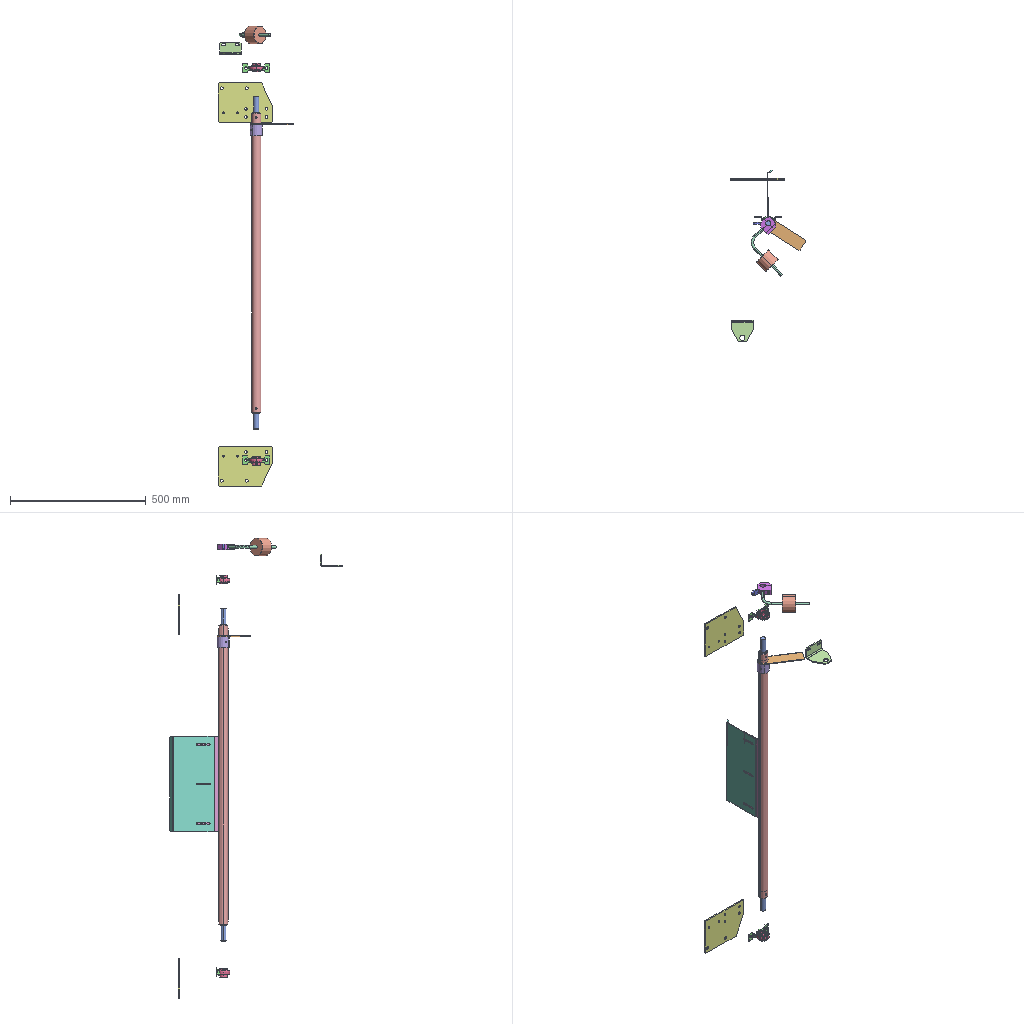Assembly | SolidWorks | 21 different items | 43 placed | box 278 x 633 x 1692 mm
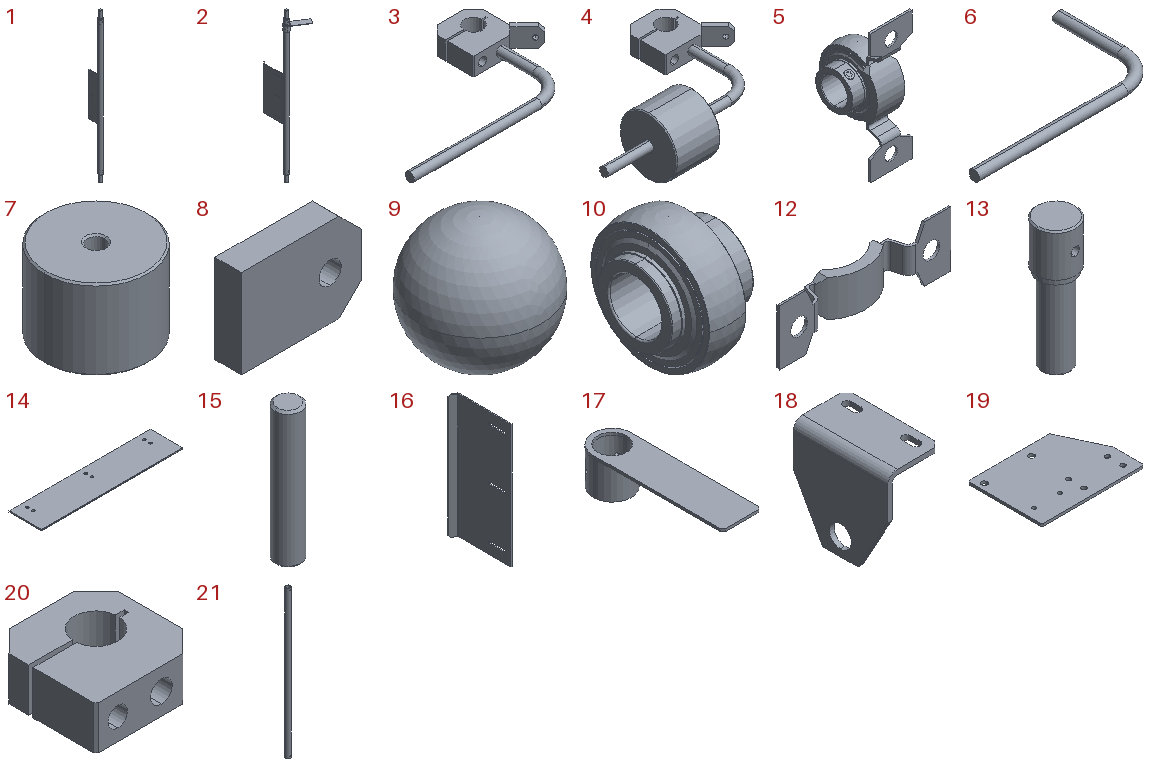Parts list (item | name | quantity | parent item | size | volume | features):
1 | (subassembly) | x1 | in 2 | 33.7 x 113.85 x 1224 mm | 469066 mm3 | -
2 | (subassembly) | x1 | - | 160.679 x 296.153 x 1224 mm | 692755 mm3 | -
3 | (subassembly) | x1 | - | 211.213 x 125 x 20 mm | 58047 mm3 | -
4 | (subassembly) | x1 | - | 211.213 x 152.5 x 65 mm | 218972 mm3 | -
5 | (subassembly) | x2 | - | 34.3 x 48.8 x 98.5 mm | 23790 mm3 | features AEMSimFeature 1
6 | - | x1 | in 4 | 175 x 96.34 x 10 mm | 19434 mm3 | features ICE 1, Sweep 1
7 | - | x1 | in 4 | 65 x 65 x 50 mm | 160925 mm3 | features Chamfer 1, Extrusion 1
8 | - | x1 | in 4 | 27 x 6 x 20 mm | 2972 mm3 | features Chamfer 1, Extrusion 1, HoleWzd 1
9 | - | x16 | in 5 | 7.938 x 7.938 x 7.938 mm | 261.898 mm3 | features BaseBody 1
10 | - | x2 | in 5 | 31 x 47 x 47 mm | 16946 mm3 | features BaseBody 1
11 | - | x2 | in 5 | - | - | features BaseBody 1
12 | - | x2 | in 5 | 98.5 x 11.15 x 32 mm | 4749 mm3 | features BaseBody 1
13 | - | x2 | in 1 | 27.9 x 27.9 x 92 mm | 37672 mm3 | features ICE 3, Chamfer 1, Extrusion 1, Fillet 1
14 | - | x1 | in 1 | 350 x 80.217 x 3 mm | 83584 mm3 | features Extrusion 1, ICE 1
15 | - | x2 | in 1 | 6 x 6 x 32 mm | 900.328 mm3 | features Chamfer 1, Extrusion 1
16 | - | x1 | in 2 | 20.321 x 162.598 x 350 mm | 177208 mm3 | features ICE 3, Fillet 2, Chamfer 1, Extrusion 1
17 | - | x1 | in 2 | 45 x 174.185 x 43 mm | 46480 mm3 | features HoleWzd 3, 3DProfileFeature 1, Chamfer 1, Extrusion 1, ICE 1
18 | - | x1 | - | 45 x 80 x 80 mm | 31465 mm3 | features ICE 3, Chamfer 2, Fillet 2, Extrusion 1, HoleWzd 1
19 | - | x2 | - | 200 x 145 x 5 mm | 133825 mm3 | features Extrusion 1
20 | - | x1 | in 4 | 50 x 50 x 20 mm | 35641 mm3 | features ICE 3, Chamfer 2, Extrusion 1, HoleWzd 1
21 | - | x1 | in 1 | 33.7 x 33.7 x 1100 mm | 308338 mm3 | features Extrusion 1, ICE 1
Mates (type | each side: item.copy, entity, surface, feature):
In the top assembly
Concentric | 13.1 face cylinder Boss-Extrude 1 | 10.1 face cylinder YAR 204-2F-28.2103002204-b(1)
Parallel | 14.1 face plane Boss-Extrude 1 | 12.1 face plane housingP 47-h(1)
Coincident | 13.1 face plane Boss-Extrude 2 | 10.1 face plane YAR 204-2F-28.2103002204-b(1)
Concentric | 13.2 face cylinder Boss-Extrude 1 | 10.2 face cylinder YAR 204-2F-28.2103002204-b(1)
Coincident | 12.1 face plane housingP 47-h(1) | 12.2 face plane housingP 47-h(1)
Coincident | 13.2 face plane Boss-Extrude 2 | 10.2 face plane YAR 204-2F-28.2103002204-b(1)
Coincident | 12.1 face plane housingP 47-h(1) | 19.1 face plane Boss-Extrude 1
Concentric | 12.1 edge | 19.1 face cylinder Boss-Extrude 1 | 2 times
Coincident | 12.2 face plane housingP 47-h(1) | 19.2 face plane Boss-Extrude 1
Concentric | 12.2 edge | 19.2 face cylinder Boss-Extrude 1
Concentric | 12.2 face cylinder housingP 47-h(1) | 19.2 face cylinder Boss-Extrude 1
Concentric | 13.1 face cylinder Boss-Extrude 1 | 20.1 face cylinder Boss-Extrude 1
Parallel | 19.1 face plane Boss-Extrude 1 | 20.1 face plane Chamfer 1
Coincident | 10.1 face plane YAR 204-2F-28.2103002204-b(1) | 20.1 face plane Boss-Extrude 1
Coincident | 19.1 face plane Boss-Extrude 1 | 18.1 face plane Boss-Extrude 1
Slot | 18.1 face plane Cut-Extrude 1 | 19.1 face cylinder Boss-Extrude 1
Slot | 18.1 face plane Cut-Extrude 2 | 19.1 face cylinder Boss-Extrude 1
In subassembly 2
Concentric | 21.1 face cylinder Boss-Extrude 1 | 17.1 face cylinder M30 ClearanceHole 1
Coincident | 14.2 face plane Boss-Extrude 1 | 16.1 face plane Boss-Extrude 1
Slot | 16.1 face cylinder Cut-Extrude 2 | 14.2 face cylinder Boss-Extrude 1 | 2 times
In subassembly 1
Concentric | 21.2 face cylinder Boss-Extrude 1 | 13.3 face cylinder Boss-Extrude 3
Concentric | 21.2 face cylinder Cut-Extrude 1 | 13.3 face cylinder Cut-Extrude 1
Concentric | 21.2 face cylinder Cut-Extrude 1 | 15.1 face cylinder Boss-Extrude 1
Coincident | 21.2 plane | 15.1 plane
Concentric | 21.2 face cylinder Boss-Extrude 1 | 13.4 face cylinder Boss-Extrude 3
Concentric | 21.2 face cylinder Cut-Extrude 1 | 15.2 face cylinder Boss-Extrude 1
Coincident | 15.1 face plane Boss-Extrude 1 | 15.2 face plane Boss-Extrude 1
Concentric | 13.4 face cylinder Cut-Extrude 1 | 15.2 face cylinder Boss-Extrude 1
Concentric | 21.2 face cylinder Boss-Extrude 1 | 14.3 face cylinder Cut-Extrude 1
Perpendicular | 14.3 face plane Boss-Extrude 1 | 1.1 plane
DistanceDim | 14.3 face plane Boss-Extrude 1 | 21.2 face plane Boss-Extrude 1
In subassembly 4
Parallel | 20.2 face plane Boss-Extrude 1 | 6.1 face plane Sweep 1
Concentric | 20.2 face cylinder Boss-Extrude 1 | 6.1 face cylinder Cut-Extrude 1
Concentric | 6.1 face cylinder Sweep 1 | 7.1 face cylinder Boss-Extrude 1
DistanceDim | 7.1 face plane Boss-Extrude 1 | 6.1 face plane Sweep 1
Coincident | 20.2 face plane Chamfer 1 | 8.1 face plane Boss-Extrude 1
Coincident | 20.2 face plane Boss-Extrude 1 | 8.1 face plane Boss-Extrude 1
DistanceDim | 8.1 edge | 20.2 edge
Concentric | 20.2 face cylinder Cut-Extrude 5 | 6.1 face cylinder Sweep 1